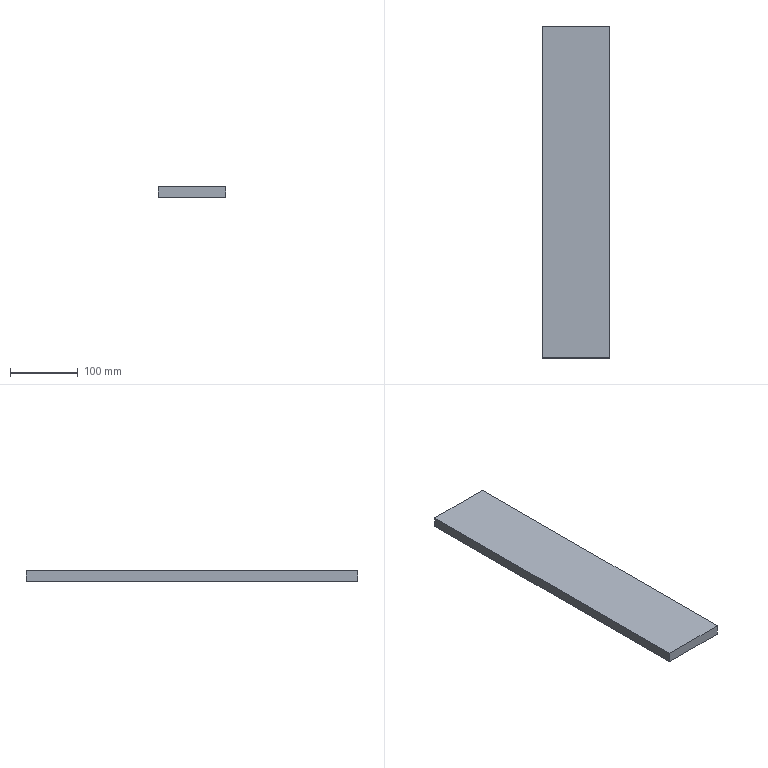Part | STEP file | Leg_left | 1 solid | 6 faces | box 100 x 490 x 15 mm | volume 735000 mm3 | plane 6
STEP:
#1=CARTESIAN_POINT('',(0.,0.,0.));
#2=DIRECTION('',(0.,0.,1.));
#3=DIRECTION('',(1.,0.,0.));
#4=AXIS2_PLACEMENT_3D('',#1,#2,#3);
#5=CARTESIAN_POINT('',(-50.,245.,-7.5));
#6=VERTEX_POINT('',#5);
#7=CARTESIAN_POINT('',(-50.,-245.,-7.5));
#8=VERTEX_POINT('',#7);
#9=CARTESIAN_POINT('',(-50.,245.,-7.5));
#10=DIRECTION('',(0.,-1.,0.));
#11=VECTOR('',#10,1.);
#12=LINE('',#9,#11);
#13=CARTESIAN_POINT('',(-50.,245.,-7.5));
#14=DIRECTION('',(0.,0.,1.));
#15=DIRECTION('',(1.,0.,0.));
#16=AXIS2_PLACEMENT_3D('',#13,#14,#15);
#17=PLANE('',#16);
#18=CARTESIAN_POINT('',(0.,0.));
#19=DIRECTION('',(0.,-1.));
#20=VECTOR('',#19,1.);
#21=LINE('',#18,#20);
#22=(GEOMETRIC_REPRESENTATION_CONTEXT(2)PARAMETRIC_REPRESENTATION_CONTEXT()REPRESENTATION_CONTEXT('',''));
#23=DEFINITIONAL_REPRESENTATION('',(#21),#22);
#24=PCURVE('',#17,#23);
#25=CARTESIAN_POINT('',(-50.,245.,7.5));
#26=DIRECTION('',(1.,0.,0.));
#27=DIRECTION('',(0.,0.,-1.));
#28=AXIS2_PLACEMENT_3D('',#25,#26,#27);
#29=PLANE('',#28);
#30=CARTESIAN_POINT('',(15.,0.));
#31=DIRECTION('',(0.,-1.));
#32=VECTOR('',#31,1.);
#33=LINE('',#30,#32);
#34=(GEOMETRIC_REPRESENTATION_CONTEXT(2)PARAMETRIC_REPRESENTATION_CONTEXT()REPRESENTATION_CONTEXT('',''));
#35=DEFINITIONAL_REPRESENTATION('',(#33),#34);
#36=PCURVE('',#29,#35);
#37=SURFACE_CURVE('',#12,(#24,#36),.PCURVE_S1.);
#38=EDGE_CURVE('',#6,#8,#37,.T.);
#39=ORIENTED_EDGE('',*,*,#38,.T.);
#40=CARTESIAN_POINT('',(50.,-245.,-7.5));
#41=VERTEX_POINT('',#40);
#42=CARTESIAN_POINT('',(-50.,-245.,-7.5));
#43=DIRECTION('',(1.,0.,0.));
#44=VECTOR('',#43,1.);
#45=LINE('',#42,#44);
#46=CARTESIAN_POINT('',(0.,-490.));
#47=DIRECTION('',(1.,0.));
#48=VECTOR('',#47,1.);
#49=LINE('',#46,#48);
#50=(GEOMETRIC_REPRESENTATION_CONTEXT(2)PARAMETRIC_REPRESENTATION_CONTEXT()REPRESENTATION_CONTEXT('',''));
#51=DEFINITIONAL_REPRESENTATION('',(#49),#50);
#52=PCURVE('',#17,#51);
#53=CARTESIAN_POINT('',(0.,-245.,0.));
#54=DIRECTION('',(0.,1.,0.));
#55=DIRECTION('',(0.,0.,1.));
#56=AXIS2_PLACEMENT_3D('',#53,#54,#55);
#57=PLANE('',#56);
#58=CARTESIAN_POINT('',(-7.5,-50.));
#59=DIRECTION('',(0.,1.));
#60=VECTOR('',#59,1.);
#61=LINE('',#58,#60);
#62=(GEOMETRIC_REPRESENTATION_CONTEXT(2)PARAMETRIC_REPRESENTATION_CONTEXT()REPRESENTATION_CONTEXT('',''));
#63=DEFINITIONAL_REPRESENTATION('',(#61),#62);
#64=PCURVE('',#57,#63);
#65=SURFACE_CURVE('',#45,(#52,#64),.PCURVE_S1.);
#66=EDGE_CURVE('',#8,#41,#65,.T.);
#67=ORIENTED_EDGE('',*,*,#66,.T.);
#68=CARTESIAN_POINT('',(50.,245.,-7.5));
#69=VERTEX_POINT('',#68);
#70=CARTESIAN_POINT('',(50.,245.,-7.5));
#71=DIRECTION('',(0.,-1.,0.));
#72=VECTOR('',#71,1.);
#73=LINE('',#70,#72);
#74=CARTESIAN_POINT('',(100.,0.));
#75=DIRECTION('',(0.,-1.));
#76=VECTOR('',#75,1.);
#77=LINE('',#74,#76);
#78=(GEOMETRIC_REPRESENTATION_CONTEXT(2)PARAMETRIC_REPRESENTATION_CONTEXT()REPRESENTATION_CONTEXT('',''));
#79=DEFINITIONAL_REPRESENTATION('',(#77),#78);
#80=PCURVE('',#17,#79);
#81=CARTESIAN_POINT('',(50.,245.,-7.5));
#82=DIRECTION('',(-1.,0.,0.));
#83=DIRECTION('',(0.,0.,1.));
#84=AXIS2_PLACEMENT_3D('',#81,#82,#83);
#85=PLANE('',#84);
#86=CARTESIAN_POINT('',(0.,0.));
#87=DIRECTION('',(0.,-1.));
#88=VECTOR('',#87,1.);
#89=LINE('',#86,#88);
#90=(GEOMETRIC_REPRESENTATION_CONTEXT(2)PARAMETRIC_REPRESENTATION_CONTEXT()REPRESENTATION_CONTEXT('',''));
#91=DEFINITIONAL_REPRESENTATION('',(#89),#90);
#92=PCURVE('',#85,#91);
#93=SURFACE_CURVE('',#73,(#80,#92),.PCURVE_S1.);
#94=EDGE_CURVE('',#69,#41,#93,.T.);
#95=ORIENTED_EDGE('',*,*,#94,.F.);
#96=CARTESIAN_POINT('',(-50.,245.,-7.5));
#97=DIRECTION('',(1.,0.,0.));
#98=VECTOR('',#97,1.);
#99=LINE('',#96,#98);
#100=CARTESIAN_POINT('',(0.,0.));
#101=DIRECTION('',(1.,0.));
#102=VECTOR('',#101,1.);
#103=LINE('',#100,#102);
#104=(GEOMETRIC_REPRESENTATION_CONTEXT(2)PARAMETRIC_REPRESENTATION_CONTEXT()REPRESENTATION_CONTEXT('',''));
#105=DEFINITIONAL_REPRESENTATION('',(#103),#104);
#106=PCURVE('',#17,#105);
#107=CARTESIAN_POINT('',(0.,245.,0.));
#108=DIRECTION('',(0.,1.,0.));
#109=DIRECTION('',(0.,0.,1.));
#110=AXIS2_PLACEMENT_3D('',#107,#108,#109);
#111=PLANE('',#110);
#112=CARTESIAN_POINT('',(-7.5,-50.));
#113=DIRECTION('',(0.,1.));
#114=VECTOR('',#113,1.);
#115=LINE('',#112,#114);
#116=(GEOMETRIC_REPRESENTATION_CONTEXT(2)PARAMETRIC_REPRESENTATION_CONTEXT()REPRESENTATION_CONTEXT('',''));
#117=DEFINITIONAL_REPRESENTATION('',(#115),#116);
#118=PCURVE('',#111,#117);
#119=SURFACE_CURVE('',#99,(#106,#118),.PCURVE_S1.);
#120=EDGE_CURVE('',#6,#69,#119,.T.);
#121=ORIENTED_EDGE('',*,*,#120,.F.);
#122=EDGE_LOOP('',(#39,#67,#95,#121));
#123=FACE_BOUND('',#122,.F.);
#124=ADVANCED_FACE('',(#123),#17,.F.);
#125=ORIENTED_EDGE('',*,*,#94,.T.);
#126=CARTESIAN_POINT('',(50.,-245.,7.5));
#127=VERTEX_POINT('',#126);
#128=CARTESIAN_POINT('',(50.,-245.,-7.5));
#129=DIRECTION('',(0.,0.,1.));
#130=VECTOR('',#129,1.);
#131=LINE('',#128,#130);
#132=CARTESIAN_POINT('',(0.,-490.));
#133=DIRECTION('',(1.,0.));
#134=VECTOR('',#133,1.);
#135=LINE('',#132,#134);
#136=(GEOMETRIC_REPRESENTATION_CONTEXT(2)PARAMETRIC_REPRESENTATION_CONTEXT()REPRESENTATION_CONTEXT('',''));
#137=DEFINITIONAL_REPRESENTATION('',(#135),#136);
#138=PCURVE('',#85,#137);
#139=CARTESIAN_POINT('',(-7.5,50.));
#140=DIRECTION('',(1.,0.));
#141=VECTOR('',#140,1.);
#142=LINE('',#139,#141);
#143=(GEOMETRIC_REPRESENTATION_CONTEXT(2)PARAMETRIC_REPRESENTATION_CONTEXT()REPRESENTATION_CONTEXT('',''));
#144=DEFINITIONAL_REPRESENTATION('',(#142),#143);
#145=PCURVE('',#57,#144);
#146=SURFACE_CURVE('',#131,(#138,#145),.PCURVE_S1.);
#147=EDGE_CURVE('',#41,#127,#146,.T.);
#148=ORIENTED_EDGE('',*,*,#147,.T.);
#149=CARTESIAN_POINT('',(50.,245.,7.5));
#150=VERTEX_POINT('',#149);
#151=CARTESIAN_POINT('',(50.,245.,7.5));
#152=DIRECTION('',(0.,-1.,0.));
#153=VECTOR('',#152,1.);
#154=LINE('',#151,#153);
#155=CARTESIAN_POINT('',(15.,0.));
#156=DIRECTION('',(0.,-1.));
#157=VECTOR('',#156,1.);
#158=LINE('',#155,#157);
#159=(GEOMETRIC_REPRESENTATION_CONTEXT(2)PARAMETRIC_REPRESENTATION_CONTEXT()REPRESENTATION_CONTEXT('',''));
#160=DEFINITIONAL_REPRESENTATION('',(#158),#159);
#161=PCURVE('',#85,#160);
#162=CARTESIAN_POINT('',(50.,245.,7.5));
#163=DIRECTION('',(0.,0.,-1.));
#164=DIRECTION('',(-1.,0.,0.));
#165=AXIS2_PLACEMENT_3D('',#162,#163,#164);
#166=PLANE('',#165);
#167=CARTESIAN_POINT('',(0.,0.));
#168=DIRECTION('',(0.,-1.));
#169=VECTOR('',#168,1.);
#170=LINE('',#167,#169);
#171=(GEOMETRIC_REPRESENTATION_CONTEXT(2)PARAMETRIC_REPRESENTATION_CONTEXT()REPRESENTATION_CONTEXT('',''));
#172=DEFINITIONAL_REPRESENTATION('',(#170),#171);
#173=PCURVE('',#166,#172);
#174=SURFACE_CURVE('',#154,(#161,#173),.PCURVE_S1.);
#175=EDGE_CURVE('',#150,#127,#174,.T.);
#176=ORIENTED_EDGE('',*,*,#175,.F.);
#177=CARTESIAN_POINT('',(50.,245.,-7.5));
#178=DIRECTION('',(0.,0.,1.));
#179=VECTOR('',#178,1.);
#180=LINE('',#177,#179);
#181=CARTESIAN_POINT('',(0.,0.));
#182=DIRECTION('',(1.,0.));
#183=VECTOR('',#182,1.);
#184=LINE('',#181,#183);
#185=(GEOMETRIC_REPRESENTATION_CONTEXT(2)PARAMETRIC_REPRESENTATION_CONTEXT()REPRESENTATION_CONTEXT('',''));
#186=DEFINITIONAL_REPRESENTATION('',(#184),#185);
#187=PCURVE('',#85,#186);
#188=CARTESIAN_POINT('',(-7.5,50.));
#189=DIRECTION('',(1.,0.));
#190=VECTOR('',#189,1.);
#191=LINE('',#188,#190);
#192=(GEOMETRIC_REPRESENTATION_CONTEXT(2)PARAMETRIC_REPRESENTATION_CONTEXT()REPRESENTATION_CONTEXT('',''));
#193=DEFINITIONAL_REPRESENTATION('',(#191),#192);
#194=PCURVE('',#111,#193);
#195=SURFACE_CURVE('',#180,(#187,#194),.PCURVE_S1.);
#196=EDGE_CURVE('',#69,#150,#195,.T.);
#197=ORIENTED_EDGE('',*,*,#196,.F.);
#198=EDGE_LOOP('',(#125,#148,#176,#197));
#199=FACE_BOUND('',#198,.F.);
#200=ADVANCED_FACE('',(#199),#85,.F.);
#201=ORIENTED_EDGE('',*,*,#175,.T.);
#202=CARTESIAN_POINT('',(-50.,-245.,7.5));
#203=VERTEX_POINT('',#202);
#204=CARTESIAN_POINT('',(50.,-245.,7.5));
#205=DIRECTION('',(-1.,0.,0.));
#206=VECTOR('',#205,1.);
#207=LINE('',#204,#206);
#208=CARTESIAN_POINT('',(0.,-490.));
#209=DIRECTION('',(1.,0.));
#210=VECTOR('',#209,1.);
#211=LINE('',#208,#210);
#212=(GEOMETRIC_REPRESENTATION_CONTEXT(2)PARAMETRIC_REPRESENTATION_CONTEXT()REPRESENTATION_CONTEXT('',''));
#213=DEFINITIONAL_REPRESENTATION('',(#211),#212);
#214=PCURVE('',#166,#213);
#215=CARTESIAN_POINT('',(7.5,50.));
#216=DIRECTION('',(0.,-1.));
#217=VECTOR('',#216,1.);
#218=LINE('',#215,#217);
#219=(GEOMETRIC_REPRESENTATION_CONTEXT(2)PARAMETRIC_REPRESENTATION_CONTEXT()REPRESENTATION_CONTEXT('',''));
#220=DEFINITIONAL_REPRESENTATION('',(#218),#219);
#221=PCURVE('',#57,#220);
#222=SURFACE_CURVE('',#207,(#214,#221),.PCURVE_S1.);
#223=EDGE_CURVE('',#127,#203,#222,.T.);
#224=ORIENTED_EDGE('',*,*,#223,.T.);
#225=CARTESIAN_POINT('',(-50.,245.,7.5));
#226=VERTEX_POINT('',#225);
#227=CARTESIAN_POINT('',(-50.,245.,7.5));
#228=DIRECTION('',(0.,-1.,0.));
#229=VECTOR('',#228,1.);
#230=LINE('',#227,#229);
#231=CARTESIAN_POINT('',(100.,0.));
#232=DIRECTION('',(0.,-1.));
#233=VECTOR('',#232,1.);
#234=LINE('',#231,#233);
#235=(GEOMETRIC_REPRESENTATION_CONTEXT(2)PARAMETRIC_REPRESENTATION_CONTEXT()REPRESENTATION_CONTEXT('',''));
#236=DEFINITIONAL_REPRESENTATION('',(#234),#235);
#237=PCURVE('',#166,#236);
#238=CARTESIAN_POINT('',(0.,0.));
#239=DIRECTION('',(0.,-1.));
#240=VECTOR('',#239,1.);
#241=LINE('',#238,#240);
#242=(GEOMETRIC_REPRESENTATION_CONTEXT(2)PARAMETRIC_REPRESENTATION_CONTEXT()REPRESENTATION_CONTEXT('',''));
#243=DEFINITIONAL_REPRESENTATION('',(#241),#242);
#244=PCURVE('',#29,#243);
#245=SURFACE_CURVE('',#230,(#237,#244),.PCURVE_S1.);
#246=EDGE_CURVE('',#226,#203,#245,.T.);
#247=ORIENTED_EDGE('',*,*,#246,.F.);
#248=CARTESIAN_POINT('',(50.,245.,7.5));
#249=DIRECTION('',(-1.,0.,0.));
#250=VECTOR('',#249,1.);
#251=LINE('',#248,#250);
#252=CARTESIAN_POINT('',(0.,0.));
#253=DIRECTION('',(1.,0.));
#254=VECTOR('',#253,1.);
#255=LINE('',#252,#254);
#256=(GEOMETRIC_REPRESENTATION_CONTEXT(2)PARAMETRIC_REPRESENTATION_CONTEXT()REPRESENTATION_CONTEXT('',''));
#257=DEFINITIONAL_REPRESENTATION('',(#255),#256);
#258=PCURVE('',#166,#257);
#259=CARTESIAN_POINT('',(7.5,50.));
#260=DIRECTION('',(0.,-1.));
#261=VECTOR('',#260,1.);
#262=LINE('',#259,#261);
#263=(GEOMETRIC_REPRESENTATION_CONTEXT(2)PARAMETRIC_REPRESENTATION_CONTEXT()REPRESENTATION_CONTEXT('',''));
#264=DEFINITIONAL_REPRESENTATION('',(#262),#263);
#265=PCURVE('',#111,#264);
#266=SURFACE_CURVE('',#251,(#258,#265),.PCURVE_S1.);
#267=EDGE_CURVE('',#150,#226,#266,.T.);
#268=ORIENTED_EDGE('',*,*,#267,.F.);
#269=EDGE_LOOP('',(#201,#224,#247,#268));
#270=FACE_BOUND('',#269,.F.);
#271=ADVANCED_FACE('',(#270),#166,.F.);
#272=ORIENTED_EDGE('',*,*,#246,.T.);
#273=CARTESIAN_POINT('',(-50.,-245.,7.5));
#274=DIRECTION('',(0.,0.,-1.));
#275=VECTOR('',#274,1.);
#276=LINE('',#273,#275);
#277=CARTESIAN_POINT('',(0.,-490.));
#278=DIRECTION('',(1.,0.));
#279=VECTOR('',#278,1.);
#280=LINE('',#277,#279);
#281=(GEOMETRIC_REPRESENTATION_CONTEXT(2)PARAMETRIC_REPRESENTATION_CONTEXT()REPRESENTATION_CONTEXT('',''));
#282=DEFINITIONAL_REPRESENTATION('',(#280),#281);
#283=PCURVE('',#29,#282);
#284=CARTESIAN_POINT('',(7.5,-50.));
#285=DIRECTION('',(-1.,0.));
#286=VECTOR('',#285,1.);
#287=LINE('',#284,#286);
#288=(GEOMETRIC_REPRESENTATION_CONTEXT(2)PARAMETRIC_REPRESENTATION_CONTEXT()REPRESENTATION_CONTEXT('',''));
#289=DEFINITIONAL_REPRESENTATION('',(#287),#288);
#290=PCURVE('',#57,#289);
#291=SURFACE_CURVE('',#276,(#283,#290),.PCURVE_S1.);
#292=EDGE_CURVE('',#203,#8,#291,.T.);
#293=ORIENTED_EDGE('',*,*,#292,.T.);
#294=ORIENTED_EDGE('',*,*,#38,.F.);
#295=CARTESIAN_POINT('',(-50.,245.,7.5));
#296=DIRECTION('',(0.,0.,-1.));
#297=VECTOR('',#296,1.);
#298=LINE('',#295,#297);
#299=CARTESIAN_POINT('',(0.,0.));
#300=DIRECTION('',(1.,0.));
#301=VECTOR('',#300,1.);
#302=LINE('',#299,#301);
#303=(GEOMETRIC_REPRESENTATION_CONTEXT(2)PARAMETRIC_REPRESENTATION_CONTEXT()REPRESENTATION_CONTEXT('',''));
#304=DEFINITIONAL_REPRESENTATION('',(#302),#303);
#305=PCURVE('',#29,#304);
#306=CARTESIAN_POINT('',(7.5,-50.));
#307=DIRECTION('',(-1.,0.));
#308=VECTOR('',#307,1.);
#309=LINE('',#306,#308);
#310=(GEOMETRIC_REPRESENTATION_CONTEXT(2)PARAMETRIC_REPRESENTATION_CONTEXT()REPRESENTATION_CONTEXT('',''));
#311=DEFINITIONAL_REPRESENTATION('',(#309),#310);
#312=PCURVE('',#111,#311);
#313=SURFACE_CURVE('',#298,(#305,#312),.PCURVE_S1.);
#314=EDGE_CURVE('',#226,#6,#313,.T.);
#315=ORIENTED_EDGE('',*,*,#314,.F.);
#316=EDGE_LOOP('',(#272,#293,#294,#315));
#317=FACE_BOUND('',#316,.F.);
#318=ADVANCED_FACE('',(#317),#29,.F.);
#319=ORIENTED_EDGE('',*,*,#120,.T.);
#320=ORIENTED_EDGE('',*,*,#196,.T.);
#321=ORIENTED_EDGE('',*,*,#267,.T.);
#322=ORIENTED_EDGE('',*,*,#314,.T.);
#323=EDGE_LOOP('',(#319,#320,#321,#322));
#324=FACE_BOUND('',#323,.F.);
#325=ADVANCED_FACE('',(#324),#111,.T.);
#326=ORIENTED_EDGE('',*,*,#66,.T.);
#327=ORIENTED_EDGE('',*,*,#147,.T.);
#328=ORIENTED_EDGE('',*,*,#223,.T.);
#329=ORIENTED_EDGE('',*,*,#292,.T.);
#330=EDGE_LOOP('',(#326,#327,#328,#329));
#331=FACE_BOUND('',#330,.T.);
#332=ADVANCED_FACE('',(#331),#57,.F.);
#333=CLOSED_SHELL('',(#124,#200,#271,#318,#325,#332));
#334=MANIFOLD_SOLID_BREP('',#333);
#335=(LENGTH_UNIT()NAMED_UNIT(*)SI_UNIT(.MILLI.,.METRE.));
#336=UNCERTAINTY_MEASURE_WITH_UNIT(LENGTH_MEASURE(0.0000001),#335,'','');
#337=(NAMED_UNIT(*)PLANE_ANGLE_UNIT()SI_UNIT($,.RADIAN.));
#338=(NAMED_UNIT(*)SI_UNIT($,.STERADIAN.)SOLID_ANGLE_UNIT());
#339=(GEOMETRIC_REPRESENTATION_CONTEXT(3)GLOBAL_UNCERTAINTY_ASSIGNED_CONTEXT((#336))GLOBAL_UNIT_ASSIGNED_CONTEXT((#335,#337,#338))REPRESENTATION_CONTEXT('',''));
#340=ADVANCED_BREP_SHAPE_REPRESENTATION('',(#4,#334),#339);